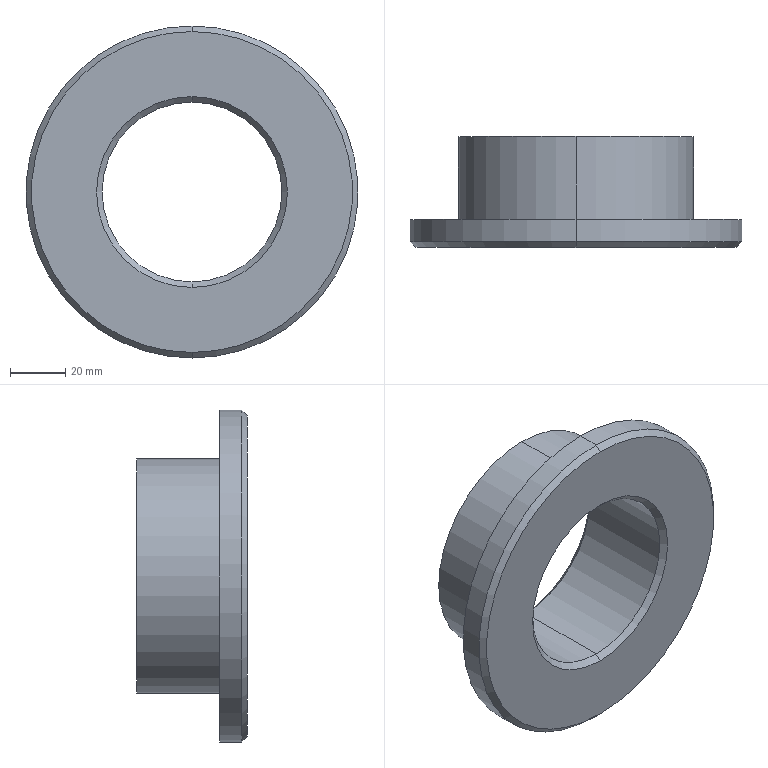Part | SolidWorks | features Chamfer 1, Revolution 1 | 1 solid | 15 faces | box 120 x 40 x 120 mm | volume 149021 mm3 | cone 6 | cylinder 6 | plane 3 | commonest cylinder face diameters 65 x2 85 x2 120 x2
STEP:
#1=CARTESIAN_POINT('',(0.,0.,-58.));
#2=VERTEX_POINT('',#1);
#3=CARTESIAN_POINT('',(0.,0.,58.));
#4=VERTEX_POINT('',#3);
#5=CARTESIAN_POINT('',(0.,0.,0.));
#6=DIRECTION('',(0.,-1.,0.));
#7=DIRECTION('',(0.,0.,1.));
#8=AXIS2_PLACEMENT_3D('',#5,#6,#7);
#9=CIRCLE('',#8,58.);
#10=EDGE_CURVE('',#2,#4,#9,.T.);
#11=ORIENTED_EDGE('',*,*,#10,.F.);
#12=CARTESIAN_POINT('',(0.,2.,-60.));
#13=VERTEX_POINT('',#12);
#14=CARTESIAN_POINT('',(0.,0.,-58.));
#15=DIRECTION('',(0.,0.7071,-0.7071));
#16=VECTOR('',#15,1000.);
#17=LINE('',#14,#16);
#18=EDGE_CURVE('',#2,#13,#17,.T.);
#19=ORIENTED_EDGE('',*,*,#18,.T.);
#20=CARTESIAN_POINT('',(0.,2.,60.));
#21=VERTEX_POINT('',#20);
#22=CARTESIAN_POINT('',(0.,2.,0.));
#23=DIRECTION('',(0.,1.,0.));
#24=DIRECTION('',(0.,0.,1.));
#25=AXIS2_PLACEMENT_3D('',#22,#23,#24);
#26=CIRCLE('',#25,60.);
#27=EDGE_CURVE('',#21,#13,#26,.T.);
#28=ORIENTED_EDGE('',*,*,#27,.F.);
#29=CARTESIAN_POINT('',(0.,0.,58.));
#30=DIRECTION('',(0.,0.7071,0.7071));
#31=VECTOR('',#30,1000.);
#32=LINE('',#29,#31);
#33=EDGE_CURVE('',#4,#21,#32,.T.);
#34=ORIENTED_EDGE('',*,*,#33,.F.);
#35=EDGE_LOOP('',(#11,#19,#28,#34));
#36=FACE_OUTER_BOUND('',#35,.T.);
#37=CARTESIAN_POINT('',(0.,0.,0.));
#38=DIRECTION('',(0.,1.,0.));
#39=DIRECTION('',(0.,0.,1.));
#40=AXIS2_PLACEMENT_3D('',#37,#38,#39);
#41=CONICAL_SURFACE('',#40,58.,0.7854);
#42=ADVANCED_FACE('',(#36),#41,.T.);
#43=CARTESIAN_POINT('',(0.,2.,32.5));
#44=VERTEX_POINT('',#43);
#45=CARTESIAN_POINT('',(0.,2.,-32.5));
#46=VERTEX_POINT('',#45);
#47=CARTESIAN_POINT('',(0.,2.,0.));
#48=DIRECTION('',(0.,-1.,0.));
#49=DIRECTION('',(0.,0.,1.));
#50=AXIS2_PLACEMENT_3D('',#47,#48,#49);
#51=CIRCLE('',#50,32.5);
#52=EDGE_CURVE('',#44,#46,#51,.T.);
#53=ORIENTED_EDGE('',*,*,#52,.F.);
#54=CARTESIAN_POINT('',(0.,0.,34.5));
#55=VERTEX_POINT('',#54);
#56=CARTESIAN_POINT('',(0.,2.,32.5));
#57=DIRECTION('',(0.,-0.7071,0.7071));
#58=VECTOR('',#57,1000.);
#59=LINE('',#56,#58);
#60=EDGE_CURVE('',#44,#55,#59,.T.);
#61=ORIENTED_EDGE('',*,*,#60,.T.);
#62=CARTESIAN_POINT('',(0.,0.,-34.5));
#63=VERTEX_POINT('',#62);
#64=CARTESIAN_POINT('',(0.,0.,0.));
#65=DIRECTION('',(0.,1.,0.));
#66=DIRECTION('',(0.,0.,1.));
#67=AXIS2_PLACEMENT_3D('',#64,#65,#66);
#68=CIRCLE('',#67,34.5);
#69=EDGE_CURVE('',#63,#55,#68,.T.);
#70=ORIENTED_EDGE('',*,*,#69,.F.);
#71=CARTESIAN_POINT('',(0.,2.,-32.5));
#72=DIRECTION('',(0.,-0.7071,-0.7071));
#73=VECTOR('',#72,1000.);
#74=LINE('',#71,#73);
#75=EDGE_CURVE('',#46,#63,#74,.T.);
#76=ORIENTED_EDGE('',*,*,#75,.F.);
#77=EDGE_LOOP('',(#53,#61,#70,#76));
#78=FACE_OUTER_BOUND('',#77,.T.);
#79=CARTESIAN_POINT('',(0.,2.,0.));
#80=DIRECTION('',(0.,-1.,0.));
#81=DIRECTION('',(0.,0.,-1.));
#82=AXIS2_PLACEMENT_3D('',#79,#80,#81);
#83=CONICAL_SURFACE('',#82,32.5,0.7854);
#84=ADVANCED_FACE('',(#78),#83,.F.);
#85=CARTESIAN_POINT('',(0.,38.,-32.5));
#86=VERTEX_POINT('',#85);
#87=CARTESIAN_POINT('',(0.,38.,32.5));
#88=VERTEX_POINT('',#87);
#89=CARTESIAN_POINT('',(0.,38.,0.));
#90=DIRECTION('',(0.,1.,0.));
#91=DIRECTION('',(0.,0.,-1.));
#92=AXIS2_PLACEMENT_3D('',#89,#90,#91);
#93=CIRCLE('',#92,32.5);
#94=EDGE_CURVE('',#86,#88,#93,.T.);
#95=ORIENTED_EDGE('',*,*,#94,.F.);
#96=CARTESIAN_POINT('',(0.,40.,-34.5));
#97=VERTEX_POINT('',#96);
#98=CARTESIAN_POINT('',(0.,40.,-34.5));
#99=DIRECTION('',(0.,0.7071,-0.7071));
#100=VECTOR('',#99,1000.);
#101=LINE('',#98,#100);
#102=EDGE_CURVE('',#86,#97,#101,.T.);
#103=ORIENTED_EDGE('',*,*,#102,.T.);
#104=CARTESIAN_POINT('',(0.,40.,34.5));
#105=VERTEX_POINT('',#104);
#106=CARTESIAN_POINT('',(0.,40.,0.));
#107=DIRECTION('',(0.,-1.,0.));
#108=DIRECTION('',(0.,0.,-1.));
#109=AXIS2_PLACEMENT_3D('',#106,#107,#108);
#110=CIRCLE('',#109,34.5);
#111=EDGE_CURVE('',#105,#97,#110,.T.);
#112=ORIENTED_EDGE('',*,*,#111,.F.);
#113=CARTESIAN_POINT('',(0.,40.,34.5));
#114=DIRECTION('',(0.,0.7071,0.7071));
#115=VECTOR('',#114,1000.);
#116=LINE('',#113,#115);
#117=EDGE_CURVE('',#88,#105,#116,.T.);
#118=ORIENTED_EDGE('',*,*,#117,.F.);
#119=EDGE_LOOP('',(#95,#103,#112,#118));
#120=FACE_OUTER_BOUND('',#119,.T.);
#121=CARTESIAN_POINT('',(0.,40.,0.));
#122=DIRECTION('',(0.,1.,0.));
#123=DIRECTION('',(0.,0.,1.));
#124=AXIS2_PLACEMENT_3D('',#121,#122,#123);
#125=CONICAL_SURFACE('',#124,34.5,0.7854);
#126=ADVANCED_FACE('',(#120),#125,.F.);
#127=CARTESIAN_POINT('',(0.,10.,-60.));
#128=VERTEX_POINT('',#127);
#129=CARTESIAN_POINT('',(0.,10.,60.));
#130=VERTEX_POINT('',#129);
#131=CARTESIAN_POINT('',(0.,10.,0.));
#132=DIRECTION('',(0.,-1.,0.));
#133=DIRECTION('',(0.,0.,-1.));
#134=AXIS2_PLACEMENT_3D('',#131,#132,#133);
#135=CIRCLE('',#134,60.);
#136=EDGE_CURVE('',#128,#130,#135,.T.);
#137=ORIENTED_EDGE('',*,*,#136,.T.);
#138=CARTESIAN_POINT('',(0.,0.,60.));
#139=DIRECTION('',(0.,-1.,0.));
#140=VECTOR('',#139,1000.);
#141=LINE('',#138,#140);
#142=EDGE_CURVE('',#130,#21,#141,.T.);
#143=ORIENTED_EDGE('',*,*,#142,.T.);
#144=ORIENTED_EDGE('',*,*,#27,.T.);
#145=CARTESIAN_POINT('',(0.,0.,-60.));
#146=DIRECTION('',(0.,-1.,0.));
#147=VECTOR('',#146,1000.);
#148=LINE('',#145,#147);
#149=EDGE_CURVE('',#128,#13,#148,.T.);
#150=ORIENTED_EDGE('',*,*,#149,.F.);
#151=EDGE_LOOP('',(#137,#143,#144,#150));
#152=FACE_OUTER_BOUND('',#151,.T.);
#153=CARTESIAN_POINT('',(0.,0.,0.));
#154=DIRECTION('',(0.,-1.,0.));
#155=DIRECTION('',(0.,0.,-1.));
#156=AXIS2_PLACEMENT_3D('',#153,#154,#155);
#157=CYLINDRICAL_SURFACE('',#156,60.);
#158=ADVANCED_FACE('',(#152),#157,.T.);
#159=CARTESIAN_POINT('',(0.,40.,-42.5));
#160=VERTEX_POINT('',#159);
#161=CARTESIAN_POINT('',(0.,40.,42.5));
#162=VERTEX_POINT('',#161);
#163=CARTESIAN_POINT('',(0.,40.,0.));
#164=DIRECTION('',(0.,-1.,0.));
#165=DIRECTION('',(0.,0.,-1.));
#166=AXIS2_PLACEMENT_3D('',#163,#164,#165);
#167=CIRCLE('',#166,42.5);
#168=EDGE_CURVE('',#160,#162,#167,.T.);
#169=ORIENTED_EDGE('',*,*,#168,.T.);
#170=CARTESIAN_POINT('',(0.,10.,42.5));
#171=VERTEX_POINT('',#170);
#172=CARTESIAN_POINT('',(0.,0.,42.5));
#173=DIRECTION('',(0.,-1.,0.));
#174=VECTOR('',#173,1000.);
#175=LINE('',#172,#174);
#176=EDGE_CURVE('',#162,#171,#175,.T.);
#177=ORIENTED_EDGE('',*,*,#176,.T.);
#178=CARTESIAN_POINT('',(0.,10.,-42.5));
#179=VERTEX_POINT('',#178);
#180=CARTESIAN_POINT('',(0.,10.,0.));
#181=DIRECTION('',(0.,-1.,0.));
#182=DIRECTION('',(0.,0.,-1.));
#183=AXIS2_PLACEMENT_3D('',#180,#181,#182);
#184=CIRCLE('',#183,42.5);
#185=EDGE_CURVE('',#179,#171,#184,.T.);
#186=ORIENTED_EDGE('',*,*,#185,.F.);
#187=CARTESIAN_POINT('',(0.,0.,-42.5));
#188=DIRECTION('',(0.,-1.,0.));
#189=VECTOR('',#188,1000.);
#190=LINE('',#187,#189);
#191=EDGE_CURVE('',#160,#179,#190,.T.);
#192=ORIENTED_EDGE('',*,*,#191,.F.);
#193=EDGE_LOOP('',(#169,#177,#186,#192));
#194=FACE_OUTER_BOUND('',#193,.T.);
#195=CARTESIAN_POINT('',(0.,0.,0.));
#196=DIRECTION('',(0.,-1.,0.));
#197=DIRECTION('',(0.,0.,-1.));
#198=AXIS2_PLACEMENT_3D('',#195,#196,#197);
#199=CYLINDRICAL_SURFACE('',#198,42.5);
#200=ADVANCED_FACE('',(#194),#199,.T.);
#201=ORIENTED_EDGE('',*,*,#94,.T.);
#202=CARTESIAN_POINT('',(0.,0.,32.5));
#203=DIRECTION('',(0.,-1.,0.));
#204=VECTOR('',#203,1000.);
#205=LINE('',#202,#204);
#206=EDGE_CURVE('',#88,#44,#205,.T.);
#207=ORIENTED_EDGE('',*,*,#206,.T.);
#208=ORIENTED_EDGE('',*,*,#52,.T.);
#209=CARTESIAN_POINT('',(0.,0.,-32.5));
#210=DIRECTION('',(0.,-1.,0.));
#211=VECTOR('',#210,1000.);
#212=LINE('',#209,#211);
#213=EDGE_CURVE('',#86,#46,#212,.T.);
#214=ORIENTED_EDGE('',*,*,#213,.F.);
#215=EDGE_LOOP('',(#201,#207,#208,#214));
#216=FACE_OUTER_BOUND('',#215,.T.);
#217=CARTESIAN_POINT('',(0.,0.,0.));
#218=DIRECTION('',(0.,-1.,0.));
#219=DIRECTION('',(0.,0.,-1.));
#220=AXIS2_PLACEMENT_3D('',#217,#218,#219);
#221=CYLINDRICAL_SURFACE('',#220,32.5);
#222=ADVANCED_FACE('',(#216),#221,.F.);
#223=ORIENTED_EDGE('',*,*,#69,.T.);
#224=CARTESIAN_POINT('',(0.,0.,0.));
#225=DIRECTION('',(0.,1.,0.));
#226=DIRECTION('',(0.,0.,1.));
#227=AXIS2_PLACEMENT_3D('',#224,#225,#226);
#228=CIRCLE('',#227,34.5);
#229=EDGE_CURVE('',#55,#63,#228,.T.);
#230=ORIENTED_EDGE('',*,*,#229,.T.);
#231=EDGE_LOOP('',(#223,#230));
#232=FACE_BOUND('',#231,.T.);
#233=CARTESIAN_POINT('',(0.,0.,0.));
#234=DIRECTION('',(0.,-1.,0.));
#235=DIRECTION('',(0.,0.,1.));
#236=AXIS2_PLACEMENT_3D('',#233,#234,#235);
#237=CIRCLE('',#236,58.);
#238=EDGE_CURVE('',#4,#2,#237,.T.);
#239=ORIENTED_EDGE('',*,*,#238,.T.);
#240=ORIENTED_EDGE('',*,*,#10,.T.);
#241=EDGE_LOOP('',(#239,#240));
#242=FACE_OUTER_BOUND('',#241,.T.);
#243=CARTESIAN_POINT('',(-60.,0.,0.));
#244=DIRECTION('',(0.,1.,0.));
#245=DIRECTION('',(0.,0.,1.));
#246=AXIS2_PLACEMENT_3D('',#243,#244,#245);
#247=PLANE('',#246);
#248=ADVANCED_FACE('',(#232,#242),#247,.F.);
#249=ORIENTED_EDGE('',*,*,#206,.F.);
#250=CARTESIAN_POINT('',(0.,38.,0.));
#251=DIRECTION('',(0.,1.,0.));
#252=DIRECTION('',(0.,0.,-1.));
#253=AXIS2_PLACEMENT_3D('',#250,#251,#252);
#254=CIRCLE('',#253,32.5);
#255=EDGE_CURVE('',#88,#86,#254,.T.);
#256=ORIENTED_EDGE('',*,*,#255,.T.);
#257=ORIENTED_EDGE('',*,*,#213,.T.);
#258=CARTESIAN_POINT('',(0.,2.,0.));
#259=DIRECTION('',(0.,-1.,0.));
#260=DIRECTION('',(0.,0.,1.));
#261=AXIS2_PLACEMENT_3D('',#258,#259,#260);
#262=CIRCLE('',#261,32.5);
#263=EDGE_CURVE('',#46,#44,#262,.T.);
#264=ORIENTED_EDGE('',*,*,#263,.T.);
#265=EDGE_LOOP('',(#249,#256,#257,#264));
#266=FACE_OUTER_BOUND('',#265,.T.);
#267=CARTESIAN_POINT('',(0.,0.,0.));
#268=DIRECTION('',(0.,-1.,0.));
#269=DIRECTION('',(0.,0.,-1.));
#270=AXIS2_PLACEMENT_3D('',#267,#268,#269);
#271=CYLINDRICAL_SURFACE('',#270,32.5);
#272=ADVANCED_FACE('',(#266),#271,.F.);
#273=ORIENTED_EDGE('',*,*,#111,.T.);
#274=CARTESIAN_POINT('',(0.,40.,0.));
#275=DIRECTION('',(0.,-1.,0.));
#276=DIRECTION('',(0.,0.,-1.));
#277=AXIS2_PLACEMENT_3D('',#274,#275,#276);
#278=CIRCLE('',#277,34.5);
#279=EDGE_CURVE('',#97,#105,#278,.T.);
#280=ORIENTED_EDGE('',*,*,#279,.T.);
#281=EDGE_LOOP('',(#273,#280));
#282=FACE_BOUND('',#281,.T.);
#283=ORIENTED_EDGE('',*,*,#168,.F.);
#284=CARTESIAN_POINT('',(0.,40.,0.));
#285=DIRECTION('',(0.,-1.,0.));
#286=DIRECTION('',(0.,0.,-1.));
#287=AXIS2_PLACEMENT_3D('',#284,#285,#286);
#288=CIRCLE('',#287,42.5);
#289=EDGE_CURVE('',#162,#160,#288,.T.);
#290=ORIENTED_EDGE('',*,*,#289,.F.);
#291=EDGE_LOOP('',(#283,#290));
#292=FACE_OUTER_BOUND('',#291,.T.);
#293=CARTESIAN_POINT('',(-32.5,40.,0.));
#294=DIRECTION('',(0.,-1.,0.));
#295=DIRECTION('',(0.,0.,-1.));
#296=AXIS2_PLACEMENT_3D('',#293,#294,#295);
#297=PLANE('',#296);
#298=ADVANCED_FACE('',(#282,#292),#297,.F.);
#299=ORIENTED_EDGE('',*,*,#176,.F.);
#300=ORIENTED_EDGE('',*,*,#289,.T.);
#301=ORIENTED_EDGE('',*,*,#191,.T.);
#302=CARTESIAN_POINT('',(0.,10.,0.));
#303=DIRECTION('',(0.,-1.,0.));
#304=DIRECTION('',(0.,0.,-1.));
#305=AXIS2_PLACEMENT_3D('',#302,#303,#304);
#306=CIRCLE('',#305,42.5);
#307=EDGE_CURVE('',#171,#179,#306,.T.);
#308=ORIENTED_EDGE('',*,*,#307,.F.);
#309=EDGE_LOOP('',(#299,#300,#301,#308));
#310=FACE_OUTER_BOUND('',#309,.T.);
#311=CARTESIAN_POINT('',(0.,0.,0.));
#312=DIRECTION('',(0.,-1.,0.));
#313=DIRECTION('',(0.,0.,-1.));
#314=AXIS2_PLACEMENT_3D('',#311,#312,#313);
#315=CYLINDRICAL_SURFACE('',#314,42.5);
#316=ADVANCED_FACE('',(#310),#315,.T.);
#317=ORIENTED_EDGE('',*,*,#136,.F.);
#318=CARTESIAN_POINT('',(0.,10.,0.));
#319=DIRECTION('',(0.,-1.,0.));
#320=DIRECTION('',(0.,0.,-1.));
#321=AXIS2_PLACEMENT_3D('',#318,#319,#320);
#322=CIRCLE('',#321,60.);
#323=EDGE_CURVE('',#130,#128,#322,.T.);
#324=ORIENTED_EDGE('',*,*,#323,.F.);
#325=EDGE_LOOP('',(#317,#324));
#326=FACE_OUTER_BOUND('',#325,.T.);
#327=ORIENTED_EDGE('',*,*,#185,.T.);
#328=ORIENTED_EDGE('',*,*,#307,.T.);
#329=EDGE_LOOP('',(#327,#328));
#330=FACE_BOUND('',#329,.T.);
#331=CARTESIAN_POINT('',(-42.5,10.,0.));
#332=DIRECTION('',(0.,-1.,0.));
#333=DIRECTION('',(0.,0.,-1.));
#334=AXIS2_PLACEMENT_3D('',#331,#332,#333);
#335=PLANE('',#334);
#336=ADVANCED_FACE('',(#326,#330),#335,.F.);
#337=ORIENTED_EDGE('',*,*,#142,.F.);
#338=ORIENTED_EDGE('',*,*,#323,.T.);
#339=ORIENTED_EDGE('',*,*,#149,.T.);
#340=CARTESIAN_POINT('',(0.,2.,0.));
#341=DIRECTION('',(0.,1.,0.));
#342=DIRECTION('',(0.,0.,1.));
#343=AXIS2_PLACEMENT_3D('',#340,#341,#342);
#344=CIRCLE('',#343,60.);
#345=EDGE_CURVE('',#13,#21,#344,.T.);
#346=ORIENTED_EDGE('',*,*,#345,.T.);
#347=EDGE_LOOP('',(#337,#338,#339,#346));
#348=FACE_OUTER_BOUND('',#347,.T.);
#349=CARTESIAN_POINT('',(0.,0.,0.));
#350=DIRECTION('',(0.,-1.,0.));
#351=DIRECTION('',(0.,0.,-1.));
#352=AXIS2_PLACEMENT_3D('',#349,#350,#351);
#353=CYLINDRICAL_SURFACE('',#352,60.);
#354=ADVANCED_FACE('',(#348),#353,.T.);
#355=ORIENTED_EDGE('',*,*,#102,.F.);
#356=ORIENTED_EDGE('',*,*,#255,.F.);
#357=ORIENTED_EDGE('',*,*,#117,.T.);
#358=ORIENTED_EDGE('',*,*,#279,.F.);
#359=EDGE_LOOP('',(#355,#356,#357,#358));
#360=FACE_OUTER_BOUND('',#359,.T.);
#361=CARTESIAN_POINT('',(0.,40.,0.));
#362=DIRECTION('',(0.,1.,0.));
#363=DIRECTION('',(0.,0.,1.));
#364=AXIS2_PLACEMENT_3D('',#361,#362,#363);
#365=CONICAL_SURFACE('',#364,34.5,0.7854);
#366=ADVANCED_FACE('',(#360),#365,.F.);
#367=ORIENTED_EDGE('',*,*,#60,.F.);
#368=ORIENTED_EDGE('',*,*,#263,.F.);
#369=ORIENTED_EDGE('',*,*,#75,.T.);
#370=ORIENTED_EDGE('',*,*,#229,.F.);
#371=EDGE_LOOP('',(#367,#368,#369,#370));
#372=FACE_OUTER_BOUND('',#371,.T.);
#373=CARTESIAN_POINT('',(0.,2.,0.));
#374=DIRECTION('',(0.,-1.,0.));
#375=DIRECTION('',(0.,0.,-1.));
#376=AXIS2_PLACEMENT_3D('',#373,#374,#375);
#377=CONICAL_SURFACE('',#376,32.5,0.7854);
#378=ADVANCED_FACE('',(#372),#377,.F.);
#379=ORIENTED_EDGE('',*,*,#18,.F.);
#380=ORIENTED_EDGE('',*,*,#238,.F.);
#381=ORIENTED_EDGE('',*,*,#33,.T.);
#382=ORIENTED_EDGE('',*,*,#345,.F.);
#383=EDGE_LOOP('',(#379,#380,#381,#382));
#384=FACE_OUTER_BOUND('',#383,.T.);
#385=CARTESIAN_POINT('',(0.,0.,0.));
#386=DIRECTION('',(0.,1.,0.));
#387=DIRECTION('',(0.,0.,1.));
#388=AXIS2_PLACEMENT_3D('',#385,#386,#387);
#389=CONICAL_SURFACE('',#388,58.,0.7854);
#390=ADVANCED_FACE('',(#384),#389,.T.);
#391=CLOSED_SHELL('',(#42,#84,#126,#158,#200,#222,#248,#272,#298,#316,#336,#354,#366,#378,#390));
#392=MANIFOLD_SOLID_BREP('',#391);
#393=CARTESIAN_POINT('',(0.,0.,0.));
#394=DIRECTION('',(0.,0.,1.));
#395=DIRECTION('',(1.,0.,0.));
#396=AXIS2_PLACEMENT_3D('',#393,#394,#395);
#397=(LENGTH_UNIT()NAMED_UNIT(*)SI_UNIT(.MILLI.,.METRE.));
#398=UNCERTAINTY_MEASURE_WITH_UNIT(LENGTH_MEASURE(0.00001),#397,'','');
#399=(NAMED_UNIT(*)PLANE_ANGLE_UNIT()SI_UNIT($,.RADIAN.));
#400=(NAMED_UNIT(*)SI_UNIT($,.STERADIAN.)SOLID_ANGLE_UNIT());
#401=(GEOMETRIC_REPRESENTATION_CONTEXT(3)GLOBAL_UNCERTAINTY_ASSIGNED_CONTEXT((#398))GLOBAL_UNIT_ASSIGNED_CONTEXT((#397,#399,#400))REPRESENTATION_CONTEXT('',''));
#402=ADVANCED_BREP_SHAPE_REPRESENTATION('',(#392,#396),#401);